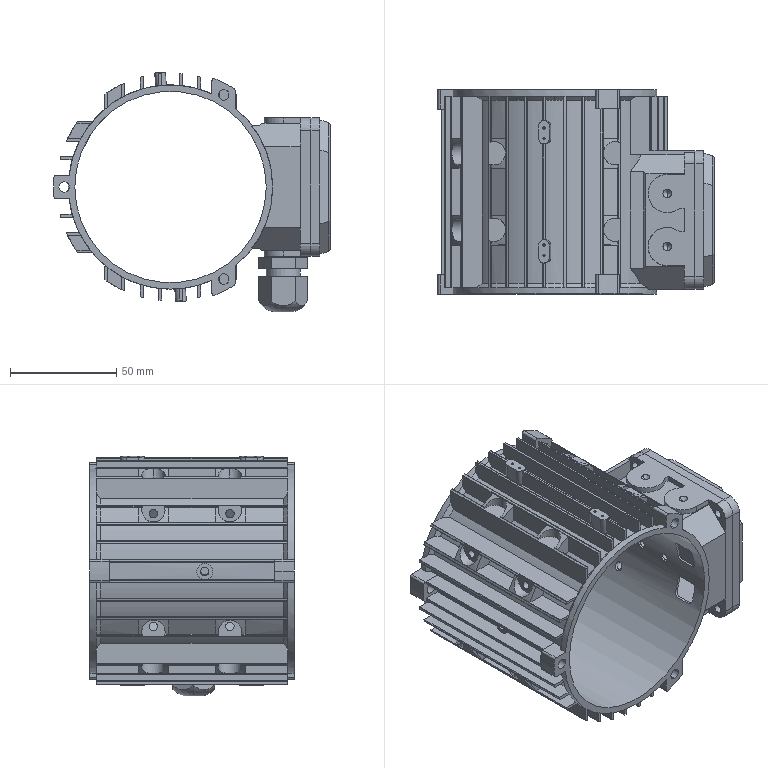Part | SolidWorks | 7 solids | 867 faces | box 130.2 x 96 x 112.64 mm | volume 107441 mm3 | plane 394 | cylinder 379 | cone 92 | torus 2 | commonest cylinder face diameters 0.4 x88 4 x60 107 x60 92 x46 5 x20 11 x18